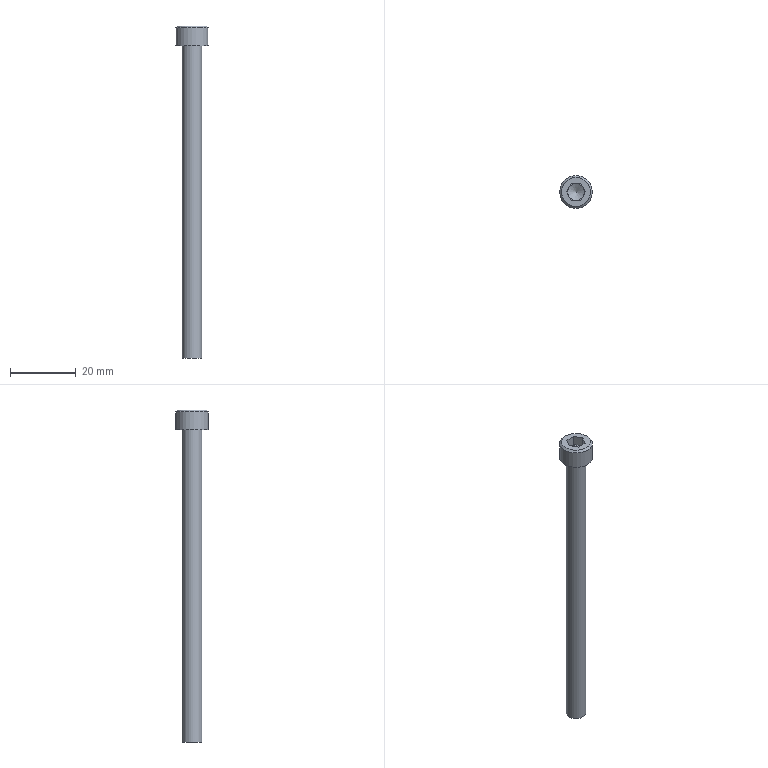Part | NX | features 5003_345_CB6-95 2 | 1 solid | 19 faces | box 10 x 10 x 101 mm | volume 3077 mm3 | plane 15 | cylinder 2 | cone 2 | commonest cylinder face diameters 6 x1 10 x1
STEP:
#1=CARTESIAN_POINT('',(136.525,24.3,-97.9));
#2=VERTEX_POINT('',#1);
#3=CARTESIAN_POINT('',(136.525,19.9,-97.9));
#4=DIRECTION('',(0.,0.,-1.));
#5=DIRECTION('',(0.,1.,0.));
#6=AXIS2_PLACEMENT_3D('',#3,#4,#5);
#7=CIRCLE('',#6,4.4);
#8=EDGE_CURVE('',#2,#2,#7,.F.);
#9=ORIENTED_EDGE('',*,*,#8,.T.);
#10=EDGE_LOOP('',(#9));
#11=FACE_BOUND('',#10,.T.);
#12=CARTESIAN_POINT('',(133.638,19.9,-97.9));
#13=VERTEX_POINT('',#12);
#14=CARTESIAN_POINT('',(135.082,17.4,-97.9));
#15=VERTEX_POINT('',#14);
#16=CARTESIAN_POINT('',(133.638,19.9,-97.9));
#17=DIRECTION('',(0.5,-0.866,0.));
#18=VECTOR('',#17,1000.);
#19=LINE('',#16,#18);
#20=EDGE_CURVE('',#13,#15,#19,.T.);
#21=ORIENTED_EDGE('',*,*,#20,.F.);
#22=CARTESIAN_POINT('',(135.082,22.4,-97.9));
#23=VERTEX_POINT('',#22);
#24=CARTESIAN_POINT('',(135.082,22.4,-97.9));
#25=DIRECTION('',(-0.5,-0.866,0.));
#26=VECTOR('',#25,1000.);
#27=LINE('',#24,#26);
#28=EDGE_CURVE('',#23,#13,#27,.T.);
#29=ORIENTED_EDGE('',*,*,#28,.F.);
#30=CARTESIAN_POINT('',(137.968,22.4,-97.9));
#31=VERTEX_POINT('',#30);
#32=CARTESIAN_POINT('',(137.968,22.4,-97.9));
#33=DIRECTION('',(-1.,0.,0.));
#34=VECTOR('',#33,1000.);
#35=LINE('',#32,#34);
#36=EDGE_CURVE('',#31,#23,#35,.T.);
#37=ORIENTED_EDGE('',*,*,#36,.F.);
#38=CARTESIAN_POINT('',(139.412,19.9,-97.9));
#39=VERTEX_POINT('',#38);
#40=CARTESIAN_POINT('',(139.412,19.9,-97.9));
#41=DIRECTION('',(-0.5,0.866,0.));
#42=VECTOR('',#41,1000.);
#43=LINE('',#40,#42);
#44=EDGE_CURVE('',#39,#31,#43,.T.);
#45=ORIENTED_EDGE('',*,*,#44,.F.);
#46=CARTESIAN_POINT('',(137.968,17.4,-97.9));
#47=VERTEX_POINT('',#46);
#48=CARTESIAN_POINT('',(137.968,17.4,-97.9));
#49=DIRECTION('',(0.5,0.866,0.));
#50=VECTOR('',#49,1000.);
#51=LINE('',#48,#50);
#52=EDGE_CURVE('',#47,#39,#51,.T.);
#53=ORIENTED_EDGE('',*,*,#52,.F.);
#54=CARTESIAN_POINT('',(135.082,17.4,-97.9));
#55=DIRECTION('',(1.,0.,0.));
#56=VECTOR('',#55,1000.);
#57=LINE('',#54,#56);
#58=EDGE_CURVE('',#15,#47,#57,.T.);
#59=ORIENTED_EDGE('',*,*,#58,.F.);
#60=EDGE_LOOP('',(#21,#29,#37,#45,#53,#59));
#61=FACE_BOUND('',#60,.T.);
#62=CARTESIAN_POINT('',(141.525,19.9,-97.9));
#63=DIRECTION('',(0.,0.,-1.));
#64=DIRECTION('',(0.,1.,0.));
#65=AXIS2_PLACEMENT_3D('',#62,#63,#64);
#66=PLANE('',#65);
#67=ADVANCED_FACE('',(#11,#61),#66,.F.);
#68=CARTESIAN_POINT('',(136.525,16.9,-198.9));
#69=VERTEX_POINT('',#68);
#70=CARTESIAN_POINT('',(136.525,19.9,-198.9));
#71=DIRECTION('',(0.,0.,1.));
#72=DIRECTION('',(0.,-1.,0.));
#73=AXIS2_PLACEMENT_3D('',#70,#71,#72);
#74=CIRCLE('',#73,3.);
#75=EDGE_CURVE('',#69,#69,#74,.T.);
#76=ORIENTED_EDGE('',*,*,#75,.F.);
#77=EDGE_LOOP('',(#76));
#78=FACE_BOUND('',#77,.T.);
#79=CARTESIAN_POINT('',(136.525,19.9,-198.9));
#80=DIRECTION('',(0.,0.,1.));
#81=DIRECTION('',(0.,-1.,0.));
#82=AXIS2_PLACEMENT_3D('',#79,#80,#81);
#83=PLANE('',#82);
#84=ADVANCED_FACE('',(#78),#83,.F.);
#85=CARTESIAN_POINT('',(136.525,16.9,-103.9));
#86=VERTEX_POINT('',#85);
#87=CARTESIAN_POINT('',(136.525,19.9,-103.9));
#88=DIRECTION('',(0.,0.,1.));
#89=DIRECTION('',(0.,-1.,0.));
#90=AXIS2_PLACEMENT_3D('',#87,#88,#89);
#91=CIRCLE('',#90,3.);
#92=EDGE_CURVE('',#86,#86,#91,.T.);
#93=ORIENTED_EDGE('',*,*,#92,.F.);
#94=EDGE_LOOP('',(#93));
#95=FACE_BOUND('',#94,.T.);
#96=ORIENTED_EDGE('',*,*,#75,.T.);
#97=EDGE_LOOP('',(#96));
#98=FACE_BOUND('',#97,.T.);
#99=CARTESIAN_POINT('',(136.525,19.9,-97.9));
#100=DIRECTION('',(0.,0.,1.));
#101=DIRECTION('',(0.,-1.,0.));
#102=AXIS2_PLACEMENT_3D('',#99,#100,#101);
#103=CYLINDRICAL_SURFACE('',#102,3.);
#104=ADVANCED_FACE('',(#95,#98),#103,.T.);
#105=CARTESIAN_POINT('',(136.525,14.9,-103.9));
#106=VERTEX_POINT('',#105);
#107=CARTESIAN_POINT('',(136.525,19.9,-103.9));
#108=DIRECTION('',(0.,0.,1.));
#109=DIRECTION('',(0.,-1.,0.));
#110=AXIS2_PLACEMENT_3D('',#107,#108,#109);
#111=CIRCLE('',#110,5.);
#112=EDGE_CURVE('',#106,#106,#111,.T.);
#113=ORIENTED_EDGE('',*,*,#112,.F.);
#114=EDGE_LOOP('',(#113));
#115=FACE_BOUND('',#114,.T.);
#116=ORIENTED_EDGE('',*,*,#92,.T.);
#117=EDGE_LOOP('',(#116));
#118=FACE_BOUND('',#117,.T.);
#119=CARTESIAN_POINT('',(139.525,19.9,-103.9));
#120=DIRECTION('',(0.,0.,1.));
#121=DIRECTION('',(0.,-1.,0.));
#122=AXIS2_PLACEMENT_3D('',#119,#120,#121);
#123=PLANE('',#122);
#124=ADVANCED_FACE('',(#115,#118),#123,.F.);
#125=CARTESIAN_POINT('',(136.525,24.9,-98.5));
#126=VERTEX_POINT('',#125);
#127=CARTESIAN_POINT('',(136.525,19.9,-98.5));
#128=DIRECTION('',(0.,0.,-1.));
#129=DIRECTION('',(0.,1.,0.));
#130=AXIS2_PLACEMENT_3D('',#127,#128,#129);
#131=CIRCLE('',#130,5.);
#132=EDGE_CURVE('',#126,#126,#131,.T.);
#133=ORIENTED_EDGE('',*,*,#132,.T.);
#134=EDGE_LOOP('',(#133));
#135=FACE_BOUND('',#134,.T.);
#136=ORIENTED_EDGE('',*,*,#112,.T.);
#137=EDGE_LOOP('',(#136));
#138=FACE_BOUND('',#137,.T.);
#139=CARTESIAN_POINT('',(136.525,19.9,-97.9));
#140=DIRECTION('',(0.,0.,1.));
#141=DIRECTION('',(0.,-1.,0.));
#142=AXIS2_PLACEMENT_3D('',#139,#140,#141);
#143=CYLINDRICAL_SURFACE('',#142,5.);
#144=ADVANCED_FACE('',(#135,#138),#143,.T.);
#145=ORIENTED_EDGE('',*,*,#132,.F.);
#146=EDGE_LOOP('',(#145));
#147=FACE_BOUND('',#146,.T.);
#148=ORIENTED_EDGE('',*,*,#8,.F.);
#149=EDGE_LOOP('',(#148));
#150=FACE_BOUND('',#149,.T.);
#151=CARTESIAN_POINT('',(136.525,19.9,-97.9));
#152=DIRECTION('',(0.,0.,-1.));
#153=DIRECTION('',(0.,1.,0.));
#154=AXIS2_PLACEMENT_3D('',#151,#152,#153);
#155=CONICAL_SURFACE('',#154,4.4,0.7854);
#156=ADVANCED_FACE('',(#147,#150),#155,.T.);
#157=CARTESIAN_POINT('',(135.082,22.4,-100.9));
#158=VERTEX_POINT('',#157);
#159=CARTESIAN_POINT('',(134.36,21.15,-100.9));
#160=VERTEX_POINT('',#159);
#161=CARTESIAN_POINT('',(135.082,22.4,-100.9));
#162=DIRECTION('',(-0.5,-0.866,0.));
#163=VECTOR('',#162,1000.);
#164=LINE('',#161,#163);
#165=EDGE_CURVE('',#158,#160,#164,.T.);
#166=ORIENTED_EDGE('',*,*,#165,.F.);
#167=CARTESIAN_POINT('',(135.082,22.4,-100.9));
#168=DIRECTION('',(0.,0.,1.));
#169=VECTOR('',#168,1000.);
#170=LINE('',#167,#169);
#171=EDGE_CURVE('',#158,#23,#170,.T.);
#172=ORIENTED_EDGE('',*,*,#171,.T.);
#173=ORIENTED_EDGE('',*,*,#28,.T.);
#174=CARTESIAN_POINT('',(133.638,19.9,-100.9));
#175=VERTEX_POINT('',#174);
#176=CARTESIAN_POINT('',(133.638,19.9,-100.9));
#177=DIRECTION('',(0.,0.,1.));
#178=VECTOR('',#177,1000.);
#179=LINE('',#176,#178);
#180=EDGE_CURVE('',#175,#13,#179,.T.);
#181=ORIENTED_EDGE('',*,*,#180,.F.);
#182=CARTESIAN_POINT('',(135.082,22.4,-100.9));
#183=DIRECTION('',(-0.5,-0.866,0.));
#184=VECTOR('',#183,1000.);
#185=LINE('',#182,#184);
#186=EDGE_CURVE('',#160,#175,#185,.T.);
#187=ORIENTED_EDGE('',*,*,#186,.F.);
#188=EDGE_LOOP('',(#166,#172,#173,#181,#187));
#189=FACE_BOUND('',#188,.T.);
#190=CARTESIAN_POINT('',(135.082,22.4,-100.9));
#191=DIRECTION('',(-0.866,0.5,0.));
#192=DIRECTION('',(0.5,0.866,0.));
#193=AXIS2_PLACEMENT_3D('',#190,#191,#192);
#194=PLANE('',#193);
#195=ADVANCED_FACE('',(#189),#194,.F.);
#196=CARTESIAN_POINT('',(137.968,22.4,-100.9));
#197=VERTEX_POINT('',#196);
#198=CARTESIAN_POINT('',(136.525,22.4,-100.9));
#199=VERTEX_POINT('',#198);
#200=CARTESIAN_POINT('',(137.968,22.4,-100.9));
#201=DIRECTION('',(-1.,0.,0.));
#202=VECTOR('',#201,1000.);
#203=LINE('',#200,#202);
#204=EDGE_CURVE('',#197,#199,#203,.T.);
#205=ORIENTED_EDGE('',*,*,#204,.F.);
#206=CARTESIAN_POINT('',(137.968,22.4,-100.9));
#207=DIRECTION('',(0.,0.,1.));
#208=VECTOR('',#207,1000.);
#209=LINE('',#206,#208);
#210=EDGE_CURVE('',#197,#31,#209,.T.);
#211=ORIENTED_EDGE('',*,*,#210,.T.);
#212=ORIENTED_EDGE('',*,*,#36,.T.);
#213=ORIENTED_EDGE('',*,*,#171,.F.);
#214=CARTESIAN_POINT('',(137.968,22.4,-100.9));
#215=DIRECTION('',(-1.,0.,0.));
#216=VECTOR('',#215,1000.);
#217=LINE('',#214,#216);
#218=EDGE_CURVE('',#199,#158,#217,.T.);
#219=ORIENTED_EDGE('',*,*,#218,.F.);
#220=EDGE_LOOP('',(#205,#211,#212,#213,#219));
#221=FACE_BOUND('',#220,.T.);
#222=CARTESIAN_POINT('',(137.968,22.4,-100.9));
#223=DIRECTION('',(0.,1.,0.));
#224=DIRECTION('',(1.,0.,0.));
#225=AXIS2_PLACEMENT_3D('',#222,#223,#224);
#226=PLANE('',#225);
#227=ADVANCED_FACE('',(#221),#226,.F.);
#228=CARTESIAN_POINT('',(139.412,19.9,-100.9));
#229=VERTEX_POINT('',#228);
#230=CARTESIAN_POINT('',(138.69,21.15,-100.9));
#231=VERTEX_POINT('',#230);
#232=CARTESIAN_POINT('',(139.412,19.9,-100.9));
#233=DIRECTION('',(-0.5,0.866,0.));
#234=VECTOR('',#233,1000.);
#235=LINE('',#232,#234);
#236=EDGE_CURVE('',#229,#231,#235,.T.);
#237=ORIENTED_EDGE('',*,*,#236,.F.);
#238=CARTESIAN_POINT('',(139.412,19.9,-100.9));
#239=DIRECTION('',(0.,0.,1.));
#240=VECTOR('',#239,1000.);
#241=LINE('',#238,#240);
#242=EDGE_CURVE('',#229,#39,#241,.T.);
#243=ORIENTED_EDGE('',*,*,#242,.T.);
#244=ORIENTED_EDGE('',*,*,#44,.T.);
#245=ORIENTED_EDGE('',*,*,#210,.F.);
#246=CARTESIAN_POINT('',(139.412,19.9,-100.9));
#247=DIRECTION('',(-0.5,0.866,0.));
#248=VECTOR('',#247,1000.);
#249=LINE('',#246,#248);
#250=EDGE_CURVE('',#231,#197,#249,.T.);
#251=ORIENTED_EDGE('',*,*,#250,.F.);
#252=EDGE_LOOP('',(#237,#243,#244,#245,#251));
#253=FACE_BOUND('',#252,.T.);
#254=CARTESIAN_POINT('',(139.412,19.9,-100.9));
#255=DIRECTION('',(0.866,0.5,0.));
#256=DIRECTION('',(0.5,-0.866,0.));
#257=AXIS2_PLACEMENT_3D('',#254,#255,#256);
#258=PLANE('',#257);
#259=ADVANCED_FACE('',(#253),#258,.F.);
#260=CARTESIAN_POINT('',(137.968,17.4,-100.9));
#261=VERTEX_POINT('',#260);
#262=CARTESIAN_POINT('',(138.69,18.65,-100.9));
#263=VERTEX_POINT('',#262);
#264=CARTESIAN_POINT('',(137.968,17.4,-100.9));
#265=DIRECTION('',(0.5,0.866,0.));
#266=VECTOR('',#265,1000.);
#267=LINE('',#264,#266);
#268=EDGE_CURVE('',#261,#263,#267,.T.);
#269=ORIENTED_EDGE('',*,*,#268,.F.);
#270=CARTESIAN_POINT('',(137.968,17.4,-100.9));
#271=DIRECTION('',(0.,0.,1.));
#272=VECTOR('',#271,1000.);
#273=LINE('',#270,#272);
#274=EDGE_CURVE('',#261,#47,#273,.T.);
#275=ORIENTED_EDGE('',*,*,#274,.T.);
#276=ORIENTED_EDGE('',*,*,#52,.T.);
#277=ORIENTED_EDGE('',*,*,#242,.F.);
#278=CARTESIAN_POINT('',(137.968,17.4,-100.9));
#279=DIRECTION('',(0.5,0.866,0.));
#280=VECTOR('',#279,1000.);
#281=LINE('',#278,#280);
#282=EDGE_CURVE('',#263,#229,#281,.T.);
#283=ORIENTED_EDGE('',*,*,#282,.F.);
#284=EDGE_LOOP('',(#269,#275,#276,#277,#283));
#285=FACE_BOUND('',#284,.T.);
#286=CARTESIAN_POINT('',(137.968,17.4,-100.9));
#287=DIRECTION('',(0.866,-0.5,0.));
#288=DIRECTION('',(-0.5,-0.866,0.));
#289=AXIS2_PLACEMENT_3D('',#286,#287,#288);
#290=PLANE('',#289);
#291=ADVANCED_FACE('',(#285),#290,.F.);
#292=CARTESIAN_POINT('',(135.082,17.4,-100.9));
#293=VERTEX_POINT('',#292);
#294=CARTESIAN_POINT('',(136.525,17.4,-100.9));
#295=VERTEX_POINT('',#294);
#296=CARTESIAN_POINT('',(135.082,17.4,-100.9));
#297=DIRECTION('',(1.,0.,0.));
#298=VECTOR('',#297,1000.);
#299=LINE('',#296,#298);
#300=EDGE_CURVE('',#293,#295,#299,.T.);
#301=ORIENTED_EDGE('',*,*,#300,.F.);
#302=CARTESIAN_POINT('',(135.082,17.4,-100.9));
#303=DIRECTION('',(0.,0.,1.));
#304=VECTOR('',#303,1000.);
#305=LINE('',#302,#304);
#306=EDGE_CURVE('',#293,#15,#305,.T.);
#307=ORIENTED_EDGE('',*,*,#306,.T.);
#308=ORIENTED_EDGE('',*,*,#58,.T.);
#309=ORIENTED_EDGE('',*,*,#274,.F.);
#310=CARTESIAN_POINT('',(135.082,17.4,-100.9));
#311=DIRECTION('',(1.,0.,0.));
#312=VECTOR('',#311,1000.);
#313=LINE('',#310,#312);
#314=EDGE_CURVE('',#295,#261,#313,.T.);
#315=ORIENTED_EDGE('',*,*,#314,.F.);
#316=EDGE_LOOP('',(#301,#307,#308,#309,#315));
#317=FACE_BOUND('',#316,.T.);
#318=CARTESIAN_POINT('',(135.082,17.4,-100.9));
#319=DIRECTION('',(0.,-1.,0.));
#320=DIRECTION('',(0.,0.,-1.));
#321=AXIS2_PLACEMENT_3D('',#318,#319,#320);
#322=PLANE('',#321);
#323=ADVANCED_FACE('',(#317),#322,.F.);
#324=CARTESIAN_POINT('',(134.36,18.65,-100.9));
#325=VERTEX_POINT('',#324);
#326=CARTESIAN_POINT('',(133.638,19.9,-100.9));
#327=DIRECTION('',(0.5,-0.866,0.));
#328=VECTOR('',#327,1000.);
#329=LINE('',#326,#328);
#330=EDGE_CURVE('',#175,#325,#329,.T.);
#331=ORIENTED_EDGE('',*,*,#330,.F.);
#332=ORIENTED_EDGE('',*,*,#180,.T.);
#333=ORIENTED_EDGE('',*,*,#20,.T.);
#334=ORIENTED_EDGE('',*,*,#306,.F.);
#335=CARTESIAN_POINT('',(133.638,19.9,-100.9));
#336=DIRECTION('',(0.5,-0.866,0.));
#337=VECTOR('',#336,1000.);
#338=LINE('',#335,#337);
#339=EDGE_CURVE('',#325,#293,#338,.T.);
#340=ORIENTED_EDGE('',*,*,#339,.F.);
#341=EDGE_LOOP('',(#331,#332,#333,#334,#340));
#342=FACE_BOUND('',#341,.T.);
#343=CARTESIAN_POINT('',(133.638,19.9,-100.9));
#344=DIRECTION('',(-0.866,-0.5,0.));
#345=DIRECTION('',(-0.5,0.866,0.));
#346=AXIS2_PLACEMENT_3D('',#343,#344,#345);
#347=PLANE('',#346);
#348=ADVANCED_FACE('',(#342),#347,.F.);
#349=ORIENTED_EDGE('',*,*,#314,.T.);
#350=ORIENTED_EDGE('',*,*,#268,.T.);
#351=CARTESIAN_POINT('',(136.525,19.9,-100.9));
#352=DIRECTION('',(0.,0.,1.));
#353=DIRECTION('',(-1.,0.,0.));
#354=AXIS2_PLACEMENT_3D('',#351,#352,#353);
#355=CIRCLE('',#354,2.5);
#356=EDGE_CURVE('',#295,#263,#355,.T.);
#357=ORIENTED_EDGE('',*,*,#356,.F.);
#358=EDGE_LOOP('',(#349,#350,#357));
#359=FACE_BOUND('',#358,.T.);
#360=CARTESIAN_POINT('',(136.525,19.9,-100.9));
#361=DIRECTION('',(0.,0.,1.));
#362=DIRECTION('',(0.,-1.,0.));
#363=AXIS2_PLACEMENT_3D('',#360,#361,#362);
#364=PLANE('',#363);
#365=ADVANCED_FACE('',(#359),#364,.T.);
#366=ORIENTED_EDGE('',*,*,#282,.T.);
#367=ORIENTED_EDGE('',*,*,#236,.T.);
#368=CARTESIAN_POINT('',(136.525,19.9,-100.9));
#369=DIRECTION('',(0.,0.,1.));
#370=DIRECTION('',(-1.,0.,0.));
#371=AXIS2_PLACEMENT_3D('',#368,#369,#370);
#372=CIRCLE('',#371,2.5);
#373=EDGE_CURVE('',#263,#231,#372,.T.);
#374=ORIENTED_EDGE('',*,*,#373,.F.);
#375=EDGE_LOOP('',(#366,#367,#374));
#376=FACE_BOUND('',#375,.T.);
#377=CARTESIAN_POINT('',(136.525,19.9,-100.9));
#378=DIRECTION('',(0.,0.,1.));
#379=DIRECTION('',(0.,-1.,0.));
#380=AXIS2_PLACEMENT_3D('',#377,#378,#379);
#381=PLANE('',#380);
#382=ADVANCED_FACE('',(#376),#381,.T.);
#383=ORIENTED_EDGE('',*,*,#250,.T.);
#384=ORIENTED_EDGE('',*,*,#204,.T.);
#385=CARTESIAN_POINT('',(136.525,19.9,-100.9));
#386=DIRECTION('',(0.,0.,1.));
#387=DIRECTION('',(-1.,0.,0.));
#388=AXIS2_PLACEMENT_3D('',#385,#386,#387);
#389=CIRCLE('',#388,2.5);
#390=EDGE_CURVE('',#231,#199,#389,.T.);
#391=ORIENTED_EDGE('',*,*,#390,.F.);
#392=EDGE_LOOP('',(#383,#384,#391));
#393=FACE_BOUND('',#392,.T.);
#394=CARTESIAN_POINT('',(136.525,19.9,-100.9));
#395=DIRECTION('',(0.,0.,1.));
#396=DIRECTION('',(0.,-1.,0.));
#397=AXIS2_PLACEMENT_3D('',#394,#395,#396);
#398=PLANE('',#397);
#399=ADVANCED_FACE('',(#393),#398,.T.);
#400=ORIENTED_EDGE('',*,*,#218,.T.);
#401=ORIENTED_EDGE('',*,*,#165,.T.);
#402=CARTESIAN_POINT('',(136.525,19.9,-100.9));
#403=DIRECTION('',(0.,0.,1.));
#404=DIRECTION('',(-1.,0.,0.));
#405=AXIS2_PLACEMENT_3D('',#402,#403,#404);
#406=CIRCLE('',#405,2.5);
#407=EDGE_CURVE('',#199,#160,#406,.T.);
#408=ORIENTED_EDGE('',*,*,#407,.F.);
#409=EDGE_LOOP('',(#400,#401,#408));
#410=FACE_BOUND('',#409,.T.);
#411=CARTESIAN_POINT('',(136.525,19.9,-100.9));
#412=DIRECTION('',(0.,0.,1.));
#413=DIRECTION('',(0.,-1.,0.));
#414=AXIS2_PLACEMENT_3D('',#411,#412,#413);
#415=PLANE('',#414);
#416=ADVANCED_FACE('',(#410),#415,.T.);
#417=ORIENTED_EDGE('',*,*,#186,.T.);
#418=ORIENTED_EDGE('',*,*,#330,.T.);
#419=CARTESIAN_POINT('',(136.525,19.9,-100.9));
#420=DIRECTION('',(0.,0.,1.));
#421=DIRECTION('',(-1.,0.,0.));
#422=AXIS2_PLACEMENT_3D('',#419,#420,#421);
#423=CIRCLE('',#422,2.5);
#424=EDGE_CURVE('',#160,#325,#423,.T.);
#425=ORIENTED_EDGE('',*,*,#424,.F.);
#426=EDGE_LOOP('',(#417,#418,#425));
#427=FACE_BOUND('',#426,.T.);
#428=CARTESIAN_POINT('',(136.525,19.9,-100.9));
#429=DIRECTION('',(0.,0.,1.));
#430=DIRECTION('',(0.,-1.,0.));
#431=AXIS2_PLACEMENT_3D('',#428,#429,#430);
#432=PLANE('',#431);
#433=ADVANCED_FACE('',(#427),#432,.T.);
#434=ORIENTED_EDGE('',*,*,#339,.T.);
#435=ORIENTED_EDGE('',*,*,#300,.T.);
#436=CARTESIAN_POINT('',(136.525,19.9,-100.9));
#437=DIRECTION('',(0.,0.,1.));
#438=DIRECTION('',(-1.,0.,0.));
#439=AXIS2_PLACEMENT_3D('',#436,#437,#438);
#440=CIRCLE('',#439,2.5);
#441=EDGE_CURVE('',#325,#295,#440,.T.);
#442=ORIENTED_EDGE('',*,*,#441,.F.);
#443=EDGE_LOOP('',(#434,#435,#442));
#444=FACE_BOUND('',#443,.T.);
#445=CARTESIAN_POINT('',(136.525,19.9,-100.9));
#446=DIRECTION('',(0.,0.,1.));
#447=DIRECTION('',(0.,-1.,0.));
#448=AXIS2_PLACEMENT_3D('',#445,#446,#447);
#449=PLANE('',#448);
#450=ADVANCED_FACE('',(#444),#449,.T.);
#451=ORIENTED_EDGE('',*,*,#441,.T.);
#452=ORIENTED_EDGE('',*,*,#356,.T.);
#453=ORIENTED_EDGE('',*,*,#373,.T.);
#454=ORIENTED_EDGE('',*,*,#390,.T.);
#455=ORIENTED_EDGE('',*,*,#407,.T.);
#456=ORIENTED_EDGE('',*,*,#424,.T.);
#457=EDGE_LOOP('',(#451,#452,#453,#454,#455,#456));
#458=FACE_BOUND('',#457,.T.);
#459=CARTESIAN_POINT('',(136.525,19.9,-102.402));
#460=VERTEX_POINT('',#459);
#461=VERTEX_LOOP('',#460);
#462=FACE_BOUND('',#461,.T.);
#463=CARTESIAN_POINT('',(136.525,19.9,-102.402));
#464=DIRECTION('',(0.,0.,1.));
#465=DIRECTION('',(-1.,0.,0.));
#466=AXIS2_PLACEMENT_3D('',#463,#464,#465);
#467=CONICAL_SURFACE('',#466,0.,1.03);
#468=ADVANCED_FACE('',(#458,#462),#467,.F.);
#469=CLOSED_SHELL('',(#67,#84,#104,#124,#144,#156,#195,#227,#259,#291,#323,#348,#365,#382,#399,#416,#433,#450,#468));
#470=MANIFOLD_SOLID_BREP('',#469);
#471=(LENGTH_UNIT()NAMED_UNIT(*)SI_UNIT(.MILLI.,.METRE.));
#472=UNCERTAINTY_MEASURE_WITH_UNIT(LENGTH_MEASURE(0.00001),#471,'','');
#473=(NAMED_UNIT(*)PLANE_ANGLE_UNIT()SI_UNIT($,.RADIAN.));
#474=(NAMED_UNIT(*)SI_UNIT($,.STERADIAN.)SOLID_ANGLE_UNIT());
#475=(GEOMETRIC_REPRESENTATION_CONTEXT(3)GLOBAL_UNCERTAINTY_ASSIGNED_CONTEXT((#472))GLOBAL_UNIT_ASSIGNED_CONTEXT((#471,#473,#474))REPRESENTATION_CONTEXT('',''));
#476=ADVANCED_BREP_SHAPE_REPRESENTATION('',(#470),#475);